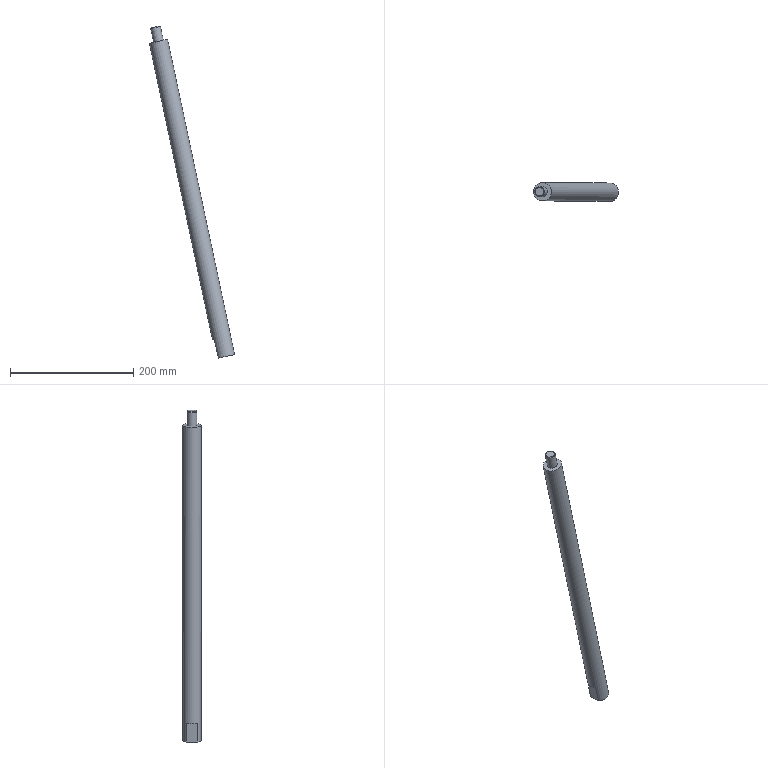Part | STEP file | solid 95 | 1 solid | 11 faces | box 137.91 x 30 x 538.185 mm | volume 371040 mm3 | plane 5 | cylinder 3 | cone 3 | commonest cylinder face diameters 10.2 x1 16 x1 30 x1